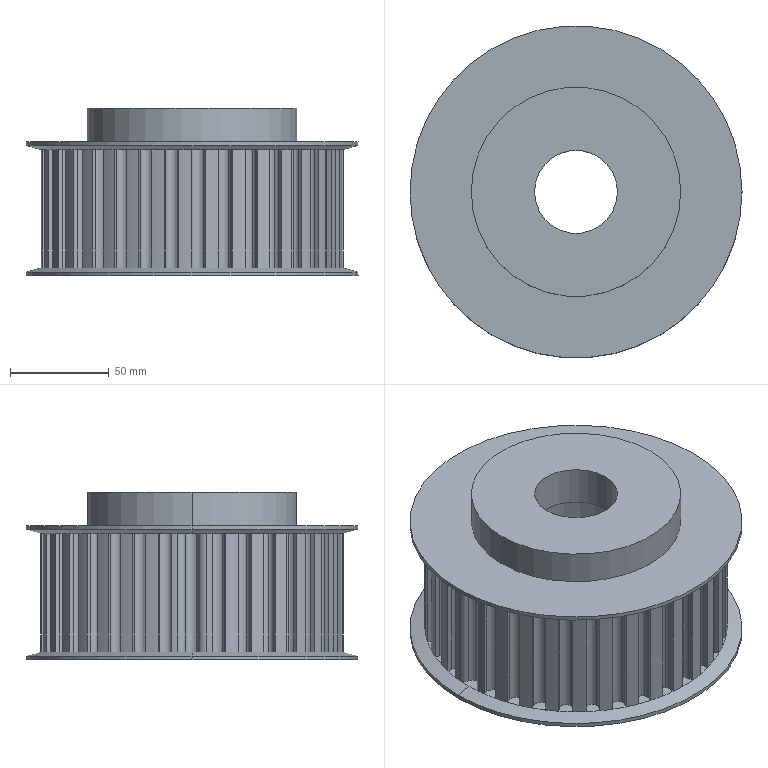Part | STEP file | LM-05-1158_default | 1 solid | 263 faces | box 168 x 168 x 85 mm | volume 1104841 mm3 | plane 142 | cylinder 115 | cone 4 | spline 2 | commonest cylinder face diameters 7 x70 153.17 x35 168 x4 42 x2 65 x2 106 x2